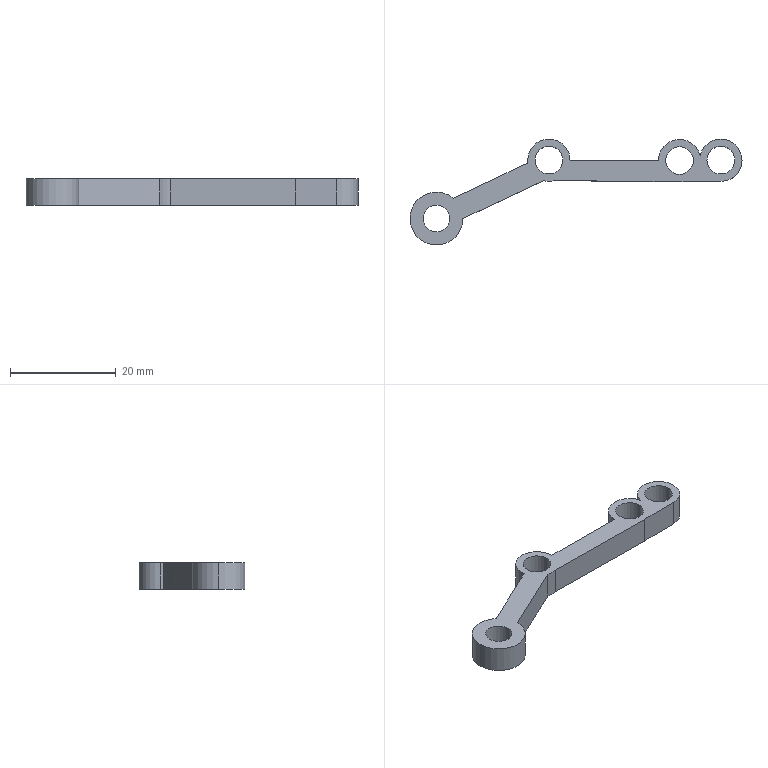Part | SolidWorks | features ICE 19, Attribute 1, Extrusion 1 | 1 solid | 27 faces | box 62.758 x 20.04 x 5 mm | volume 1442 mm3 | cylinder 18 | plane 9 | commonest cylinder face diameters 8 x7 5.25 x6 10 x3 5 x2